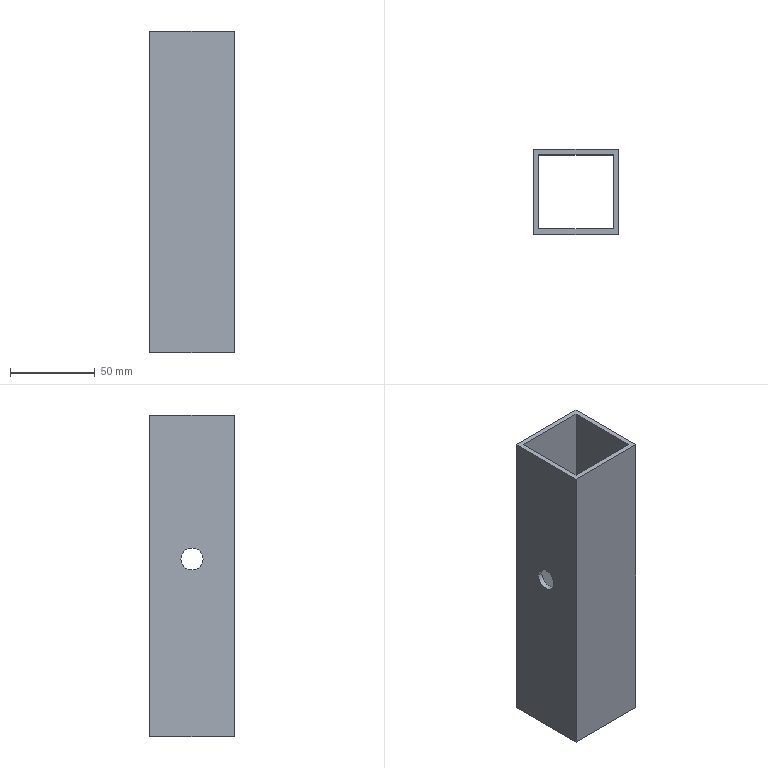Part | SolidWorks | features Cut 1, Extrusion 1 | 1 solid | 14 faces | box 50 x 50 x 190 mm | volume 106364 mm3 | plane 10 | cylinder 4 | commonest cylinder face diameters 13 x4
STEP:
#1=CARTESIAN_POINT('',(0.,-31.5,105.));
#2=VERTEX_POINT('',#1);
#3=CARTESIAN_POINT('',(0.,-18.5,105.));
#4=VERTEX_POINT('',#3);
#5=CARTESIAN_POINT('',(0.,-25.,105.));
#6=DIRECTION('',(1.,0.,0.));
#7=DIRECTION('',(0.,0.,-1.));
#8=AXIS2_PLACEMENT_3D('',#5,#6,#7);
#9=CIRCLE('',#8,6.5);
#10=EDGE_CURVE('',#2,#4,#9,.T.);
#11=ORIENTED_EDGE('',*,*,#10,.F.);
#12=CARTESIAN_POINT('',(3.,-31.5,105.));
#13=VERTEX_POINT('',#12);
#14=CARTESIAN_POINT('',(-80.,-31.5,105.));
#15=DIRECTION('',(1.,0.,0.));
#16=VECTOR('',#15,1000.);
#17=LINE('',#14,#16);
#18=EDGE_CURVE('',#2,#13,#17,.T.);
#19=ORIENTED_EDGE('',*,*,#18,.T.);
#20=CARTESIAN_POINT('',(3.,-18.5,105.));
#21=VERTEX_POINT('',#20);
#22=CARTESIAN_POINT('',(3.,-25.,105.));
#23=DIRECTION('',(1.,0.,0.));
#24=DIRECTION('',(0.,0.,-1.));
#25=AXIS2_PLACEMENT_3D('',#22,#23,#24);
#26=CIRCLE('',#25,6.5);
#27=EDGE_CURVE('',#13,#21,#26,.T.);
#28=ORIENTED_EDGE('',*,*,#27,.T.);
#29=CARTESIAN_POINT('',(-80.,-18.5,105.));
#30=DIRECTION('',(1.,0.,0.));
#31=VECTOR('',#30,1000.);
#32=LINE('',#29,#31);
#33=EDGE_CURVE('',#4,#21,#32,.T.);
#34=ORIENTED_EDGE('',*,*,#33,.F.);
#35=EDGE_LOOP('',(#11,#19,#28,#34));
#36=FACE_OUTER_BOUND('',#35,.T.);
#37=CARTESIAN_POINT('',(-80.,-25.,105.));
#38=DIRECTION('',(1.,0.,0.));
#39=DIRECTION('',(0.,1.,0.));
#40=AXIS2_PLACEMENT_3D('',#37,#38,#39);
#41=CYLINDRICAL_SURFACE('',#40,6.5);
#42=ADVANCED_FACE('',(#36),#41,.F.);
#43=CARTESIAN_POINT('',(47.,-18.5,105.));
#44=VERTEX_POINT('',#43);
#45=CARTESIAN_POINT('',(47.,-31.5,105.));
#46=VERTEX_POINT('',#45);
#47=CARTESIAN_POINT('',(47.,-25.,105.));
#48=DIRECTION('',(-1.,0.,0.));
#49=DIRECTION('',(0.,0.,1.));
#50=AXIS2_PLACEMENT_3D('',#47,#48,#49);
#51=CIRCLE('',#50,6.5);
#52=EDGE_CURVE('',#44,#46,#51,.T.);
#53=ORIENTED_EDGE('',*,*,#52,.T.);
#54=CARTESIAN_POINT('',(50.,-31.5,105.));
#55=VERTEX_POINT('',#54);
#56=CARTESIAN_POINT('',(-80.,-31.5,105.));
#57=DIRECTION('',(1.,0.,0.));
#58=VECTOR('',#57,1000.);
#59=LINE('',#56,#58);
#60=EDGE_CURVE('',#46,#55,#59,.T.);
#61=ORIENTED_EDGE('',*,*,#60,.T.);
#62=CARTESIAN_POINT('',(50.,-18.5,105.));
#63=VERTEX_POINT('',#62);
#64=CARTESIAN_POINT('',(50.,-25.,105.));
#65=DIRECTION('',(1.,0.,0.));
#66=DIRECTION('',(0.,1.,0.));
#67=AXIS2_PLACEMENT_3D('',#64,#65,#66);
#68=CIRCLE('',#67,6.5);
#69=EDGE_CURVE('',#55,#63,#68,.T.);
#70=ORIENTED_EDGE('',*,*,#69,.T.);
#71=CARTESIAN_POINT('',(-80.,-18.5,105.));
#72=DIRECTION('',(1.,0.,0.));
#73=VECTOR('',#72,1000.);
#74=LINE('',#71,#73);
#75=EDGE_CURVE('',#44,#63,#74,.T.);
#76=ORIENTED_EDGE('',*,*,#75,.F.);
#77=EDGE_LOOP('',(#53,#61,#70,#76));
#78=FACE_OUTER_BOUND('',#77,.T.);
#79=CARTESIAN_POINT('',(-80.,-25.,105.));
#80=DIRECTION('',(1.,0.,0.));
#81=DIRECTION('',(0.,1.,0.));
#82=AXIS2_PLACEMENT_3D('',#79,#80,#81);
#83=CYLINDRICAL_SURFACE('',#82,6.5);
#84=ADVANCED_FACE('',(#78),#83,.F.);
#85=CARTESIAN_POINT('',(0.,0.,190.));
#86=VERTEX_POINT('',#85);
#87=CARTESIAN_POINT('',(0.,-50.,190.));
#88=VERTEX_POINT('',#87);
#89=CARTESIAN_POINT('',(0.,-50.,190.));
#90=DIRECTION('',(0.,-1.,0.));
#91=VECTOR('',#90,1000.);
#92=LINE('',#89,#91);
#93=EDGE_CURVE('',#86,#88,#92,.T.);
#94=ORIENTED_EDGE('',*,*,#93,.T.);
#95=CARTESIAN_POINT('',(50.,-50.,190.));
#96=VERTEX_POINT('',#95);
#97=CARTESIAN_POINT('',(50.,-50.,190.));
#98=DIRECTION('',(1.,0.,0.));
#99=VECTOR('',#98,1000.);
#100=LINE('',#97,#99);
#101=EDGE_CURVE('',#88,#96,#100,.T.);
#102=ORIENTED_EDGE('',*,*,#101,.T.);
#103=CARTESIAN_POINT('',(50.,0.,190.));
#104=VERTEX_POINT('',#103);
#105=CARTESIAN_POINT('',(50.,0.,190.));
#106=DIRECTION('',(0.,1.,0.));
#107=VECTOR('',#106,1000.);
#108=LINE('',#105,#107);
#109=EDGE_CURVE('',#96,#104,#108,.T.);
#110=ORIENTED_EDGE('',*,*,#109,.T.);
#111=CARTESIAN_POINT('',(0.,0.,190.));
#112=DIRECTION('',(-1.,0.,0.));
#113=VECTOR('',#112,1000.);
#114=LINE('',#111,#113);
#115=EDGE_CURVE('',#104,#86,#114,.T.);
#116=ORIENTED_EDGE('',*,*,#115,.T.);
#117=EDGE_LOOP('',(#94,#102,#110,#116));
#118=FACE_OUTER_BOUND('',#117,.T.);
#119=CARTESIAN_POINT('',(3.,-3.,190.));
#120=VERTEX_POINT('',#119);
#121=CARTESIAN_POINT('',(3.,-47.,190.));
#122=VERTEX_POINT('',#121);
#123=CARTESIAN_POINT('',(3.,-47.,190.));
#124=DIRECTION('',(0.,-1.,0.));
#125=VECTOR('',#124,1000.);
#126=LINE('',#123,#125);
#127=EDGE_CURVE('',#120,#122,#126,.T.);
#128=ORIENTED_EDGE('',*,*,#127,.F.);
#129=CARTESIAN_POINT('',(47.,-3.,190.));
#130=VERTEX_POINT('',#129);
#131=CARTESIAN_POINT('',(3.,-3.,190.));
#132=DIRECTION('',(-1.,0.,0.));
#133=VECTOR('',#132,1000.);
#134=LINE('',#131,#133);
#135=EDGE_CURVE('',#130,#120,#134,.T.);
#136=ORIENTED_EDGE('',*,*,#135,.F.);
#137=CARTESIAN_POINT('',(47.,-47.,190.));
#138=VERTEX_POINT('',#137);
#139=CARTESIAN_POINT('',(47.,-3.,190.));
#140=DIRECTION('',(0.,1.,0.));
#141=VECTOR('',#140,1000.);
#142=LINE('',#139,#141);
#143=EDGE_CURVE('',#138,#130,#142,.T.);
#144=ORIENTED_EDGE('',*,*,#143,.F.);
#145=CARTESIAN_POINT('',(47.,-47.,190.));
#146=DIRECTION('',(1.,0.,0.));
#147=VECTOR('',#146,1000.);
#148=LINE('',#145,#147);
#149=EDGE_CURVE('',#122,#138,#148,.T.);
#150=ORIENTED_EDGE('',*,*,#149,.F.);
#151=EDGE_LOOP('',(#128,#136,#144,#150));
#152=FACE_BOUND('',#151,.T.);
#153=CARTESIAN_POINT('',(0.,0.,190.));
#154=DIRECTION('',(0.,0.,-1.));
#155=DIRECTION('',(-1.,0.,0.));
#156=AXIS2_PLACEMENT_3D('',#153,#154,#155);
#157=PLANE('',#156);
#158=ADVANCED_FACE('',(#118,#152),#157,.F.);
#159=CARTESIAN_POINT('',(0.,0.,0.));
#160=VERTEX_POINT('',#159);
#161=CARTESIAN_POINT('',(0.,-50.,0.));
#162=VERTEX_POINT('',#161);
#163=CARTESIAN_POINT('',(0.,-50.,0.));
#164=DIRECTION('',(0.,-1.,0.));
#165=VECTOR('',#164,1000.);
#166=LINE('',#163,#165);
#167=EDGE_CURVE('',#160,#162,#166,.T.);
#168=ORIENTED_EDGE('',*,*,#167,.F.);
#169=CARTESIAN_POINT('',(50.,0.,0.));
#170=VERTEX_POINT('',#169);
#171=CARTESIAN_POINT('',(0.,0.,0.));
#172=DIRECTION('',(-1.,0.,0.));
#173=VECTOR('',#172,1000.);
#174=LINE('',#171,#173);
#175=EDGE_CURVE('',#170,#160,#174,.T.);
#176=ORIENTED_EDGE('',*,*,#175,.F.);
#177=CARTESIAN_POINT('',(50.,-50.,0.));
#178=VERTEX_POINT('',#177);
#179=CARTESIAN_POINT('',(50.,0.,0.));
#180=DIRECTION('',(0.,1.,0.));
#181=VECTOR('',#180,1000.);
#182=LINE('',#179,#181);
#183=EDGE_CURVE('',#178,#170,#182,.T.);
#184=ORIENTED_EDGE('',*,*,#183,.F.);
#185=CARTESIAN_POINT('',(50.,-50.,0.));
#186=DIRECTION('',(1.,0.,0.));
#187=VECTOR('',#186,1000.);
#188=LINE('',#185,#187);
#189=EDGE_CURVE('',#162,#178,#188,.T.);
#190=ORIENTED_EDGE('',*,*,#189,.F.);
#191=EDGE_LOOP('',(#168,#176,#184,#190));
#192=FACE_OUTER_BOUND('',#191,.T.);
#193=CARTESIAN_POINT('',(47.,-3.,0.));
#194=VERTEX_POINT('',#193);
#195=CARTESIAN_POINT('',(3.,-3.,0.));
#196=VERTEX_POINT('',#195);
#197=CARTESIAN_POINT('',(3.,-3.,0.));
#198=DIRECTION('',(-1.,0.,0.));
#199=VECTOR('',#198,1000.);
#200=LINE('',#197,#199);
#201=EDGE_CURVE('',#194,#196,#200,.T.);
#202=ORIENTED_EDGE('',*,*,#201,.T.);
#203=CARTESIAN_POINT('',(3.,-47.,0.));
#204=VERTEX_POINT('',#203);
#205=CARTESIAN_POINT('',(3.,-47.,0.));
#206=DIRECTION('',(0.,-1.,0.));
#207=VECTOR('',#206,1000.);
#208=LINE('',#205,#207);
#209=EDGE_CURVE('',#196,#204,#208,.T.);
#210=ORIENTED_EDGE('',*,*,#209,.T.);
#211=CARTESIAN_POINT('',(47.,-47.,0.));
#212=VERTEX_POINT('',#211);
#213=CARTESIAN_POINT('',(47.,-47.,0.));
#214=DIRECTION('',(1.,0.,0.));
#215=VECTOR('',#214,1000.);
#216=LINE('',#213,#215);
#217=EDGE_CURVE('',#204,#212,#216,.T.);
#218=ORIENTED_EDGE('',*,*,#217,.T.);
#219=CARTESIAN_POINT('',(47.,-3.,0.));
#220=DIRECTION('',(0.,1.,0.));
#221=VECTOR('',#220,1000.);
#222=LINE('',#219,#221);
#223=EDGE_CURVE('',#212,#194,#222,.T.);
#224=ORIENTED_EDGE('',*,*,#223,.T.);
#225=EDGE_LOOP('',(#202,#210,#218,#224));
#226=FACE_BOUND('',#225,.T.);
#227=CARTESIAN_POINT('',(0.,0.,0.));
#228=DIRECTION('',(0.,0.,-1.));
#229=DIRECTION('',(-1.,0.,0.));
#230=AXIS2_PLACEMENT_3D('',#227,#228,#229);
#231=PLANE('',#230);
#232=ADVANCED_FACE('',(#192,#226),#231,.T.);
#233=CARTESIAN_POINT('',(0.,-25.,105.));
#234=DIRECTION('',(1.,0.,0.));
#235=DIRECTION('',(0.,0.,-1.));
#236=AXIS2_PLACEMENT_3D('',#233,#234,#235);
#237=CIRCLE('',#236,6.5);
#238=EDGE_CURVE('',#4,#2,#237,.T.);
#239=ORIENTED_EDGE('',*,*,#238,.T.);
#240=ORIENTED_EDGE('',*,*,#10,.T.);
#241=EDGE_LOOP('',(#239,#240));
#242=FACE_BOUND('',#241,.T.);
#243=ORIENTED_EDGE('',*,*,#167,.T.);
#244=CARTESIAN_POINT('',(0.,-50.,190.));
#245=DIRECTION('',(0.,0.,-1.));
#246=VECTOR('',#245,1000.);
#247=LINE('',#244,#246);
#248=EDGE_CURVE('',#88,#162,#247,.T.);
#249=ORIENTED_EDGE('',*,*,#248,.F.);
#250=ORIENTED_EDGE('',*,*,#93,.F.);
#251=CARTESIAN_POINT('',(0.,0.,190.));
#252=DIRECTION('',(0.,0.,-1.));
#253=VECTOR('',#252,1000.);
#254=LINE('',#251,#253);
#255=EDGE_CURVE('',#86,#160,#254,.T.);
#256=ORIENTED_EDGE('',*,*,#255,.T.);
#257=EDGE_LOOP('',(#243,#249,#250,#256));
#258=FACE_OUTER_BOUND('',#257,.T.);
#259=CARTESIAN_POINT('',(0.,-50.,190.));
#260=DIRECTION('',(1.,0.,0.));
#261=DIRECTION('',(0.,0.,-1.));
#262=AXIS2_PLACEMENT_3D('',#259,#260,#261);
#263=PLANE('',#262);
#264=ADVANCED_FACE('',(#242,#258),#263,.F.);
#265=ORIENTED_EDGE('',*,*,#189,.T.);
#266=CARTESIAN_POINT('',(50.,-50.,190.));
#267=DIRECTION('',(0.,0.,-1.));
#268=VECTOR('',#267,1000.);
#269=LINE('',#266,#268);
#270=EDGE_CURVE('',#96,#178,#269,.T.);
#271=ORIENTED_EDGE('',*,*,#270,.F.);
#272=ORIENTED_EDGE('',*,*,#101,.F.);
#273=ORIENTED_EDGE('',*,*,#248,.T.);
#274=EDGE_LOOP('',(#265,#271,#272,#273));
#275=FACE_OUTER_BOUND('',#274,.T.);
#276=CARTESIAN_POINT('',(50.,-50.,190.));
#277=DIRECTION('',(0.,1.,0.));
#278=DIRECTION('',(0.,0.,1.));
#279=AXIS2_PLACEMENT_3D('',#276,#277,#278);
#280=PLANE('',#279);
#281=ADVANCED_FACE('',(#275),#280,.F.);
#282=CARTESIAN_POINT('',(50.,-25.,105.));
#283=DIRECTION('',(1.,0.,0.));
#284=DIRECTION('',(0.,1.,0.));
#285=AXIS2_PLACEMENT_3D('',#282,#283,#284);
#286=CIRCLE('',#285,6.5);
#287=EDGE_CURVE('',#63,#55,#286,.T.);
#288=ORIENTED_EDGE('',*,*,#287,.F.);
#289=ORIENTED_EDGE('',*,*,#69,.F.);
#290=EDGE_LOOP('',(#288,#289));
#291=FACE_BOUND('',#290,.T.);
#292=ORIENTED_EDGE('',*,*,#183,.T.);
#293=CARTESIAN_POINT('',(50.,0.,190.));
#294=DIRECTION('',(0.,0.,-1.));
#295=VECTOR('',#294,1000.);
#296=LINE('',#293,#295);
#297=EDGE_CURVE('',#104,#170,#296,.T.);
#298=ORIENTED_EDGE('',*,*,#297,.F.);
#299=ORIENTED_EDGE('',*,*,#109,.F.);
#300=ORIENTED_EDGE('',*,*,#270,.T.);
#301=EDGE_LOOP('',(#292,#298,#299,#300));
#302=FACE_OUTER_BOUND('',#301,.T.);
#303=CARTESIAN_POINT('',(50.,0.,190.));
#304=DIRECTION('',(-1.,0.,0.));
#305=DIRECTION('',(0.,-1.,0.));
#306=AXIS2_PLACEMENT_3D('',#303,#304,#305);
#307=PLANE('',#306);
#308=ADVANCED_FACE('',(#291,#302),#307,.F.);
#309=ORIENTED_EDGE('',*,*,#175,.T.);
#310=ORIENTED_EDGE('',*,*,#255,.F.);
#311=ORIENTED_EDGE('',*,*,#115,.F.);
#312=ORIENTED_EDGE('',*,*,#297,.T.);
#313=EDGE_LOOP('',(#309,#310,#311,#312));
#314=FACE_OUTER_BOUND('',#313,.T.);
#315=CARTESIAN_POINT('',(0.,0.,190.));
#316=DIRECTION('',(0.,-1.,0.));
#317=DIRECTION('',(0.,0.,-1.));
#318=AXIS2_PLACEMENT_3D('',#315,#316,#317);
#319=PLANE('',#318);
#320=ADVANCED_FACE('',(#314),#319,.F.);
#321=CARTESIAN_POINT('',(3.,-25.,105.));
#322=DIRECTION('',(1.,0.,0.));
#323=DIRECTION('',(0.,0.,-1.));
#324=AXIS2_PLACEMENT_3D('',#321,#322,#323);
#325=CIRCLE('',#324,6.5);
#326=EDGE_CURVE('',#21,#13,#325,.T.);
#327=ORIENTED_EDGE('',*,*,#326,.F.);
#328=ORIENTED_EDGE('',*,*,#27,.F.);
#329=EDGE_LOOP('',(#327,#328));
#330=FACE_BOUND('',#329,.T.);
#331=ORIENTED_EDGE('',*,*,#209,.F.);
#332=CARTESIAN_POINT('',(3.,-3.,190.));
#333=DIRECTION('',(0.,0.,-1.));
#334=VECTOR('',#333,1000.);
#335=LINE('',#332,#334);
#336=EDGE_CURVE('',#120,#196,#335,.T.);
#337=ORIENTED_EDGE('',*,*,#336,.F.);
#338=ORIENTED_EDGE('',*,*,#127,.T.);
#339=CARTESIAN_POINT('',(3.,-47.,190.));
#340=DIRECTION('',(0.,0.,-1.));
#341=VECTOR('',#340,1000.);
#342=LINE('',#339,#341);
#343=EDGE_CURVE('',#122,#204,#342,.T.);
#344=ORIENTED_EDGE('',*,*,#343,.T.);
#345=EDGE_LOOP('',(#331,#337,#338,#344));
#346=FACE_OUTER_BOUND('',#345,.T.);
#347=CARTESIAN_POINT('',(3.,-47.,190.));
#348=DIRECTION('',(1.,0.,0.));
#349=DIRECTION('',(0.,0.,-1.));
#350=AXIS2_PLACEMENT_3D('',#347,#348,#349);
#351=PLANE('',#350);
#352=ADVANCED_FACE('',(#330,#346),#351,.T.);
#353=ORIENTED_EDGE('',*,*,#217,.F.);
#354=ORIENTED_EDGE('',*,*,#343,.F.);
#355=ORIENTED_EDGE('',*,*,#149,.T.);
#356=CARTESIAN_POINT('',(47.,-47.,190.));
#357=DIRECTION('',(0.,0.,-1.));
#358=VECTOR('',#357,1000.);
#359=LINE('',#356,#358);
#360=EDGE_CURVE('',#138,#212,#359,.T.);
#361=ORIENTED_EDGE('',*,*,#360,.T.);
#362=EDGE_LOOP('',(#353,#354,#355,#361));
#363=FACE_OUTER_BOUND('',#362,.T.);
#364=CARTESIAN_POINT('',(47.,-47.,190.));
#365=DIRECTION('',(0.,1.,0.));
#366=DIRECTION('',(0.,0.,1.));
#367=AXIS2_PLACEMENT_3D('',#364,#365,#366);
#368=PLANE('',#367);
#369=ADVANCED_FACE('',(#363),#368,.T.);
#370=ORIENTED_EDGE('',*,*,#52,.F.);
#371=CARTESIAN_POINT('',(47.,-25.,105.));
#372=DIRECTION('',(-1.,0.,0.));
#373=DIRECTION('',(0.,0.,1.));
#374=AXIS2_PLACEMENT_3D('',#371,#372,#373);
#375=CIRCLE('',#374,6.5);
#376=EDGE_CURVE('',#46,#44,#375,.T.);
#377=ORIENTED_EDGE('',*,*,#376,.F.);
#378=EDGE_LOOP('',(#370,#377));
#379=FACE_BOUND('',#378,.T.);
#380=ORIENTED_EDGE('',*,*,#223,.F.);
#381=ORIENTED_EDGE('',*,*,#360,.F.);
#382=ORIENTED_EDGE('',*,*,#143,.T.);
#383=CARTESIAN_POINT('',(47.,-3.,190.));
#384=DIRECTION('',(0.,0.,-1.));
#385=VECTOR('',#384,1000.);
#386=LINE('',#383,#385);
#387=EDGE_CURVE('',#130,#194,#386,.T.);
#388=ORIENTED_EDGE('',*,*,#387,.T.);
#389=EDGE_LOOP('',(#380,#381,#382,#388));
#390=FACE_OUTER_BOUND('',#389,.T.);
#391=CARTESIAN_POINT('',(47.,-3.,190.));
#392=DIRECTION('',(-1.,0.,0.));
#393=DIRECTION('',(0.,0.,1.));
#394=AXIS2_PLACEMENT_3D('',#391,#392,#393);
#395=PLANE('',#394);
#396=ADVANCED_FACE('',(#379,#390),#395,.T.);
#397=ORIENTED_EDGE('',*,*,#201,.F.);
#398=ORIENTED_EDGE('',*,*,#387,.F.);
#399=ORIENTED_EDGE('',*,*,#135,.T.);
#400=ORIENTED_EDGE('',*,*,#336,.T.);
#401=EDGE_LOOP('',(#397,#398,#399,#400));
#402=FACE_OUTER_BOUND('',#401,.T.);
#403=CARTESIAN_POINT('',(3.,-3.,190.));
#404=DIRECTION('',(0.,-1.,0.));
#405=DIRECTION('',(0.,0.,-1.));
#406=AXIS2_PLACEMENT_3D('',#403,#404,#405);
#407=PLANE('',#406);
#408=ADVANCED_FACE('',(#402),#407,.T.);
#409=ORIENTED_EDGE('',*,*,#60,.F.);
#410=ORIENTED_EDGE('',*,*,#376,.T.);
#411=ORIENTED_EDGE('',*,*,#75,.T.);
#412=ORIENTED_EDGE('',*,*,#287,.T.);
#413=EDGE_LOOP('',(#409,#410,#411,#412));
#414=FACE_OUTER_BOUND('',#413,.T.);
#415=CARTESIAN_POINT('',(-80.,-25.,105.));
#416=DIRECTION('',(1.,0.,0.));
#417=DIRECTION('',(0.,1.,0.));
#418=AXIS2_PLACEMENT_3D('',#415,#416,#417);
#419=CYLINDRICAL_SURFACE('',#418,6.5);
#420=ADVANCED_FACE('',(#414),#419,.F.);
#421=ORIENTED_EDGE('',*,*,#18,.F.);
#422=ORIENTED_EDGE('',*,*,#238,.F.);
#423=ORIENTED_EDGE('',*,*,#33,.T.);
#424=ORIENTED_EDGE('',*,*,#326,.T.);
#425=EDGE_LOOP('',(#421,#422,#423,#424));
#426=FACE_OUTER_BOUND('',#425,.T.);
#427=CARTESIAN_POINT('',(-80.,-25.,105.));
#428=DIRECTION('',(1.,0.,0.));
#429=DIRECTION('',(0.,1.,0.));
#430=AXIS2_PLACEMENT_3D('',#427,#428,#429);
#431=CYLINDRICAL_SURFACE('',#430,6.5);
#432=ADVANCED_FACE('',(#426),#431,.F.);
#433=CLOSED_SHELL('',(#42,#84,#158,#232,#264,#281,#308,#320,#352,#369,#396,#408,#420,#432));
#434=MANIFOLD_SOLID_BREP('',#433);
#435=CARTESIAN_POINT('',(0.,0.,0.));
#436=DIRECTION('',(0.,0.,1.));
#437=DIRECTION('',(1.,0.,0.));
#438=AXIS2_PLACEMENT_3D('',#435,#436,#437);
#439=(LENGTH_UNIT()NAMED_UNIT(*)SI_UNIT(.MILLI.,.METRE.));
#440=UNCERTAINTY_MEASURE_WITH_UNIT(LENGTH_MEASURE(0.00001),#439,'','');
#441=(NAMED_UNIT(*)PLANE_ANGLE_UNIT()SI_UNIT($,.RADIAN.));
#442=(NAMED_UNIT(*)SI_UNIT($,.STERADIAN.)SOLID_ANGLE_UNIT());
#443=(GEOMETRIC_REPRESENTATION_CONTEXT(3)GLOBAL_UNCERTAINTY_ASSIGNED_CONTEXT((#440))GLOBAL_UNIT_ASSIGNED_CONTEXT((#439,#441,#442))REPRESENTATION_CONTEXT('',''));
#444=ADVANCED_BREP_SHAPE_REPRESENTATION('',(#434,#438),#443);